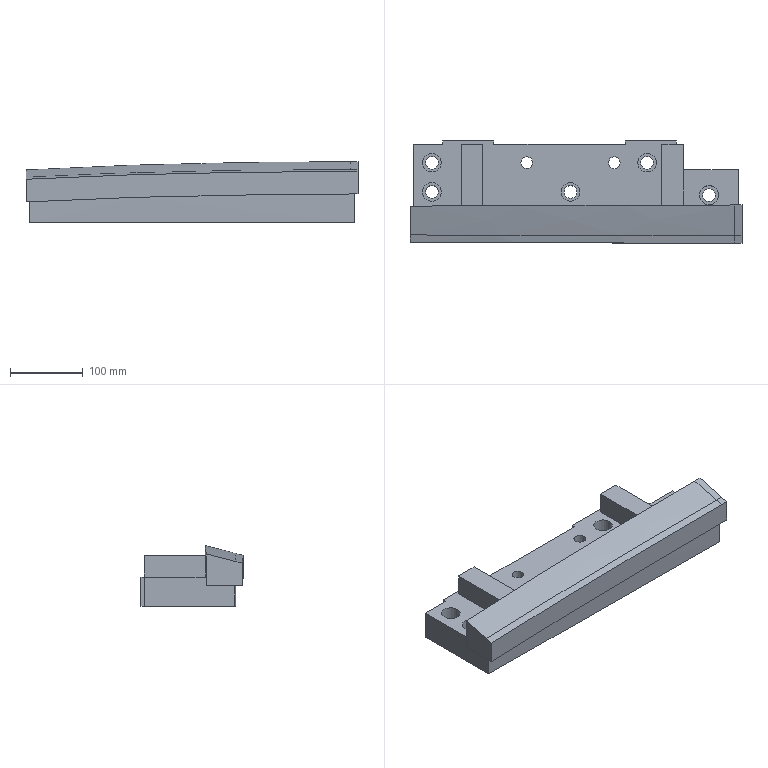Part | NX | features solid 2 | 1 solid | 49 faces | box 455 x 140.199 x 83.16 mm | volume 2999318 mm3 | plane 27 | cylinder 12 | spline 10 | commonest cylinder face diameters 17.5 x5 25.5 x4 16 x2 26 x1